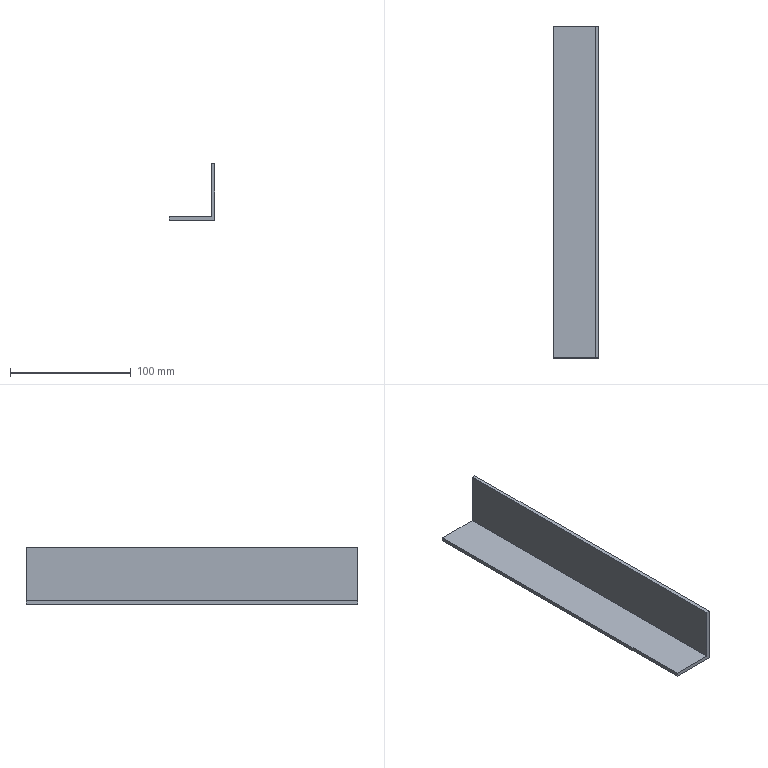Part | STEP file | Guide wheel mechanism revised.sldasm-Part-188 | 1 solid | 8 faces | box 38 x 275 x 47 mm | volume 67650 mm3 | plane 8
STEP:
#1=CARTESIAN_POINT('',(-224.,1428.01,213.));
#2=VERTEX_POINT('',#1);
#3=CARTESIAN_POINT('',(-259.,1428.01,213.));
#4=VERTEX_POINT('',#3);
#5=CARTESIAN_POINT('',(-221.,1428.01,213.));
#6=DIRECTION('',(-1.,0.,0.));
#7=VECTOR('',#6,1000.);
#8=LINE('',#5,#7);
#9=EDGE_CURVE('',#2,#4,#8,.T.);
#10=ORIENTED_EDGE('',*,*,#9,.T.);
#11=CARTESIAN_POINT('',(-259.,1428.01,210.));
#12=VERTEX_POINT('',#11);
#13=CARTESIAN_POINT('',(-259.,1428.01,210.));
#14=DIRECTION('',(0.,0.,1.));
#15=VECTOR('',#14,1000.);
#16=LINE('',#13,#15);
#17=EDGE_CURVE('',#12,#4,#16,.T.);
#18=ORIENTED_EDGE('',*,*,#17,.F.);
#19=CARTESIAN_POINT('',(-221.,1428.01,210.));
#20=VERTEX_POINT('',#19);
#21=CARTESIAN_POINT('',(-221.,1428.01,210.));
#22=DIRECTION('',(-1.,0.,0.));
#23=VECTOR('',#22,1000.);
#24=LINE('',#21,#23);
#25=EDGE_CURVE('',#20,#12,#24,.T.);
#26=ORIENTED_EDGE('',*,*,#25,.F.);
#27=CARTESIAN_POINT('',(-221.,1428.01,257.));
#28=VERTEX_POINT('',#27);
#29=CARTESIAN_POINT('',(-221.,1428.01,257.));
#30=DIRECTION('',(0.,0.,-1.));
#31=VECTOR('',#30,1000.);
#32=LINE('',#29,#31);
#33=EDGE_CURVE('',#28,#20,#32,.T.);
#34=ORIENTED_EDGE('',*,*,#33,.F.);
#35=CARTESIAN_POINT('',(-224.,1428.01,257.));
#36=VERTEX_POINT('',#35);
#37=CARTESIAN_POINT('',(-224.,1428.01,257.));
#38=DIRECTION('',(1.,0.,0.));
#39=VECTOR('',#38,1000.);
#40=LINE('',#37,#39);
#41=EDGE_CURVE('',#36,#28,#40,.T.);
#42=ORIENTED_EDGE('',*,*,#41,.F.);
#43=CARTESIAN_POINT('',(-224.,1428.01,257.));
#44=DIRECTION('',(0.,0.,-1.));
#45=VECTOR('',#44,1000.);
#46=LINE('',#43,#45);
#47=EDGE_CURVE('',#36,#2,#46,.T.);
#48=ORIENTED_EDGE('',*,*,#47,.T.);
#49=EDGE_LOOP('',(#10,#18,#26,#34,#42,#48));
#50=FACE_OUTER_BOUND('',#49,.T.);
#51=CARTESIAN_POINT('',(0.,1428.01,0.));
#52=DIRECTION('',(0.,-1.,0.));
#53=DIRECTION('',(1.,0.,0.));
#54=AXIS2_PLACEMENT_3D('',#51,#52,#53);
#55=PLANE('',#54);
#56=ADVANCED_FACE('',(#50),#55,.T.);
#57=CARTESIAN_POINT('',(-259.,1703.01,213.));
#58=VERTEX_POINT('',#57);
#59=CARTESIAN_POINT('',(-259.,1763.45,213.));
#60=DIRECTION('',(0.,-1.,0.));
#61=VECTOR('',#60,1000.);
#62=LINE('',#59,#61);
#63=EDGE_CURVE('',#58,#4,#62,.T.);
#64=ORIENTED_EDGE('',*,*,#63,.F.);
#65=CARTESIAN_POINT('',(-259.,1703.01,210.));
#66=VERTEX_POINT('',#65);
#67=CARTESIAN_POINT('',(-259.,1703.01,210.));
#68=DIRECTION('',(0.,0.,-1.));
#69=VECTOR('',#68,1000.);
#70=LINE('',#67,#69);
#71=EDGE_CURVE('',#58,#66,#70,.T.);
#72=ORIENTED_EDGE('',*,*,#71,.T.);
#73=CARTESIAN_POINT('',(-259.,1763.45,210.));
#74=DIRECTION('',(0.,-1.,0.));
#75=VECTOR('',#74,1000.);
#76=LINE('',#73,#75);
#77=EDGE_CURVE('',#66,#12,#76,.T.);
#78=ORIENTED_EDGE('',*,*,#77,.T.);
#79=ORIENTED_EDGE('',*,*,#17,.T.);
#80=EDGE_LOOP('',(#64,#72,#78,#79));
#81=FACE_OUTER_BOUND('',#80,.T.);
#82=CARTESIAN_POINT('',(-259.,1763.45,210.));
#83=DIRECTION('',(1.,0.,0.));
#84=DIRECTION('',(0.,0.,-1.));
#85=AXIS2_PLACEMENT_3D('',#82,#83,#84);
#86=PLANE('',#85);
#87=ADVANCED_FACE('',(#81),#86,.F.);
#88=ORIENTED_EDGE('',*,*,#77,.F.);
#89=CARTESIAN_POINT('',(-221.,1703.01,210.));
#90=VERTEX_POINT('',#89);
#91=CARTESIAN_POINT('',(-221.,1703.01,210.));
#92=DIRECTION('',(1.,0.,0.));
#93=VECTOR('',#92,1000.);
#94=LINE('',#91,#93);
#95=EDGE_CURVE('',#66,#90,#94,.T.);
#96=ORIENTED_EDGE('',*,*,#95,.T.);
#97=CARTESIAN_POINT('',(-221.,1763.45,210.));
#98=DIRECTION('',(0.,-1.,0.));
#99=VECTOR('',#98,1000.);
#100=LINE('',#97,#99);
#101=EDGE_CURVE('',#90,#20,#100,.T.);
#102=ORIENTED_EDGE('',*,*,#101,.T.);
#103=ORIENTED_EDGE('',*,*,#25,.T.);
#104=EDGE_LOOP('',(#88,#96,#102,#103));
#105=FACE_OUTER_BOUND('',#104,.T.);
#106=CARTESIAN_POINT('',(-221.,1763.45,210.));
#107=DIRECTION('',(0.,0.,1.));
#108=DIRECTION('',(1.,0.,0.));
#109=AXIS2_PLACEMENT_3D('',#106,#107,#108);
#110=PLANE('',#109);
#111=ADVANCED_FACE('',(#105),#110,.F.);
#112=ORIENTED_EDGE('',*,*,#101,.F.);
#113=CARTESIAN_POINT('',(-221.,1703.01,257.));
#114=VERTEX_POINT('',#113);
#115=CARTESIAN_POINT('',(-221.,1703.01,257.));
#116=DIRECTION('',(0.,0.,1.));
#117=VECTOR('',#116,1000.);
#118=LINE('',#115,#117);
#119=EDGE_CURVE('',#90,#114,#118,.T.);
#120=ORIENTED_EDGE('',*,*,#119,.T.);
#121=CARTESIAN_POINT('',(-221.,1763.45,257.));
#122=DIRECTION('',(0.,-1.,0.));
#123=VECTOR('',#122,1000.);
#124=LINE('',#121,#123);
#125=EDGE_CURVE('',#114,#28,#124,.T.);
#126=ORIENTED_EDGE('',*,*,#125,.T.);
#127=ORIENTED_EDGE('',*,*,#33,.T.);
#128=EDGE_LOOP('',(#112,#120,#126,#127));
#129=FACE_OUTER_BOUND('',#128,.T.);
#130=CARTESIAN_POINT('',(-221.,1763.45,257.));
#131=DIRECTION('',(-1.,0.,0.));
#132=DIRECTION('',(0.,0.,1.));
#133=AXIS2_PLACEMENT_3D('',#130,#131,#132);
#134=PLANE('',#133);
#135=ADVANCED_FACE('',(#129),#134,.F.);
#136=ORIENTED_EDGE('',*,*,#125,.F.);
#137=CARTESIAN_POINT('',(-224.,1703.01,257.));
#138=VERTEX_POINT('',#137);
#139=CARTESIAN_POINT('',(-224.,1703.01,257.));
#140=DIRECTION('',(-1.,0.,0.));
#141=VECTOR('',#140,1000.);
#142=LINE('',#139,#141);
#143=EDGE_CURVE('',#114,#138,#142,.T.);
#144=ORIENTED_EDGE('',*,*,#143,.T.);
#145=CARTESIAN_POINT('',(-224.,1763.45,257.));
#146=DIRECTION('',(0.,-1.,0.));
#147=VECTOR('',#146,1000.);
#148=LINE('',#145,#147);
#149=EDGE_CURVE('',#138,#36,#148,.T.);
#150=ORIENTED_EDGE('',*,*,#149,.T.);
#151=ORIENTED_EDGE('',*,*,#41,.T.);
#152=EDGE_LOOP('',(#136,#144,#150,#151));
#153=FACE_OUTER_BOUND('',#152,.T.);
#154=CARTESIAN_POINT('',(-224.,1763.45,257.));
#155=DIRECTION('',(0.,0.,-1.));
#156=DIRECTION('',(-1.,0.,0.));
#157=AXIS2_PLACEMENT_3D('',#154,#155,#156);
#158=PLANE('',#157);
#159=ADVANCED_FACE('',(#153),#158,.F.);
#160=CARTESIAN_POINT('',(-224.,1703.01,213.));
#161=VERTEX_POINT('',#160);
#162=CARTESIAN_POINT('',(-224.,1703.01,257.));
#163=DIRECTION('',(0.,0.,1.));
#164=VECTOR('',#163,1000.);
#165=LINE('',#162,#164);
#166=EDGE_CURVE('',#161,#138,#165,.T.);
#167=ORIENTED_EDGE('',*,*,#166,.F.);
#168=CARTESIAN_POINT('',(-224.,1763.45,213.));
#169=DIRECTION('',(0.,-1.,0.));
#170=VECTOR('',#169,1000.);
#171=LINE('',#168,#170);
#172=EDGE_CURVE('',#161,#2,#171,.T.);
#173=ORIENTED_EDGE('',*,*,#172,.T.);
#174=ORIENTED_EDGE('',*,*,#47,.F.);
#175=ORIENTED_EDGE('',*,*,#149,.F.);
#176=EDGE_LOOP('',(#167,#173,#174,#175));
#177=FACE_OUTER_BOUND('',#176,.T.);
#178=CARTESIAN_POINT('',(-224.,1763.45,257.));
#179=DIRECTION('',(-1.,0.,0.));
#180=DIRECTION('',(0.,0.,1.));
#181=AXIS2_PLACEMENT_3D('',#178,#179,#180);
#182=PLANE('',#181);
#183=ADVANCED_FACE('',(#177),#182,.T.);
#184=CARTESIAN_POINT('',(-221.,1703.01,213.));
#185=DIRECTION('',(1.,0.,0.));
#186=VECTOR('',#185,1000.);
#187=LINE('',#184,#186);
#188=EDGE_CURVE('',#58,#161,#187,.T.);
#189=ORIENTED_EDGE('',*,*,#188,.F.);
#190=ORIENTED_EDGE('',*,*,#63,.T.);
#191=ORIENTED_EDGE('',*,*,#9,.F.);
#192=ORIENTED_EDGE('',*,*,#172,.F.);
#193=EDGE_LOOP('',(#189,#190,#191,#192));
#194=FACE_OUTER_BOUND('',#193,.T.);
#195=CARTESIAN_POINT('',(-221.,1763.45,213.));
#196=DIRECTION('',(0.,0.,1.));
#197=DIRECTION('',(1.,0.,0.));
#198=AXIS2_PLACEMENT_3D('',#195,#196,#197);
#199=PLANE('',#198);
#200=ADVANCED_FACE('',(#194),#199,.T.);
#201=ORIENTED_EDGE('',*,*,#188,.T.);
#202=ORIENTED_EDGE('',*,*,#166,.T.);
#203=ORIENTED_EDGE('',*,*,#143,.F.);
#204=ORIENTED_EDGE('',*,*,#119,.F.);
#205=ORIENTED_EDGE('',*,*,#95,.F.);
#206=ORIENTED_EDGE('',*,*,#71,.F.);
#207=EDGE_LOOP('',(#201,#202,#203,#204,#205,#206));
#208=FACE_OUTER_BOUND('',#207,.T.);
#209=CARTESIAN_POINT('',(-221.,1703.01,257.));
#210=DIRECTION('',(0.,-1.,0.));
#211=DIRECTION('',(0.,0.,-1.));
#212=AXIS2_PLACEMENT_3D('',#209,#210,#211);
#213=PLANE('',#212);
#214=ADVANCED_FACE('',(#208),#213,.F.);
#215=CLOSED_SHELL('',(#56,#87,#111,#135,#159,#183,#200,#214));
#216=MANIFOLD_SOLID_BREP('',#215);
#217=CARTESIAN_POINT('',(0.,0.,0.));
#218=DIRECTION('',(0.,0.,1.));
#219=DIRECTION('',(1.,0.,0.));
#220=AXIS2_PLACEMENT_3D('',#217,#218,#219);
#221=(LENGTH_UNIT()NAMED_UNIT(*)SI_UNIT(.MILLI.,.METRE.));
#222=UNCERTAINTY_MEASURE_WITH_UNIT(LENGTH_MEASURE(0.00001),#221,'','');
#223=(NAMED_UNIT(*)PLANE_ANGLE_UNIT()SI_UNIT($,.RADIAN.));
#224=(NAMED_UNIT(*)SI_UNIT($,.STERADIAN.)SOLID_ANGLE_UNIT());
#225=(GEOMETRIC_REPRESENTATION_CONTEXT(3)GLOBAL_UNCERTAINTY_ASSIGNED_CONTEXT((#222))GLOBAL_UNIT_ASSIGNED_CONTEXT((#221,#223,#224))REPRESENTATION_CONTEXT('',''));
#226=ADVANCED_BREP_SHAPE_REPRESENTATION('',(#216,#220),#225);